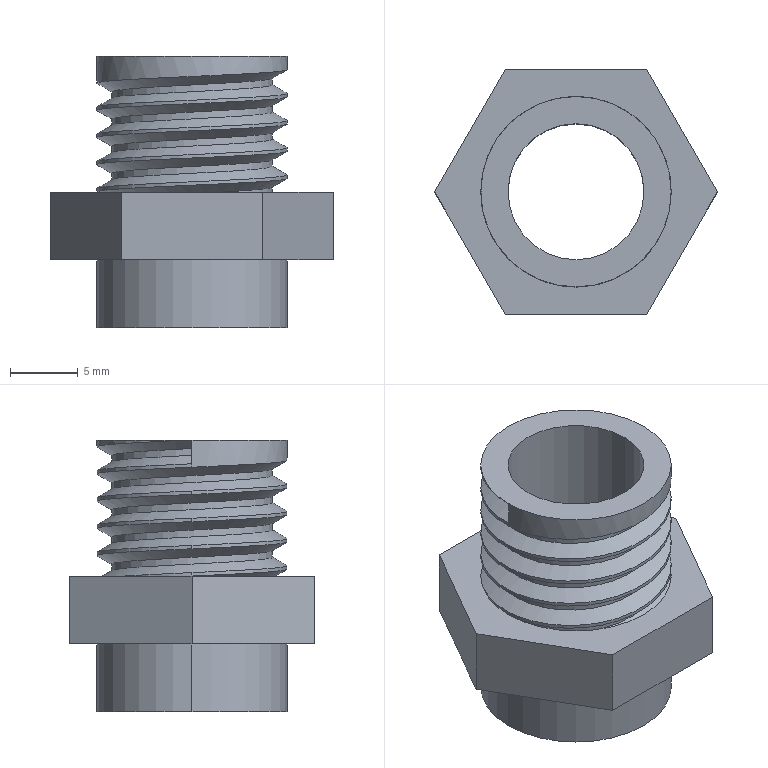Part | SolidWorks | features ICE 2, Extrusion 1, SweepThread 1 | 1 solid | 32 faces | box 20.785 x 18 x 20 mm | volume 1890 mm3 | cylinder 17 | plane 12 | spline 3 | commonest cylinder face diameters 14 x15 10 x2